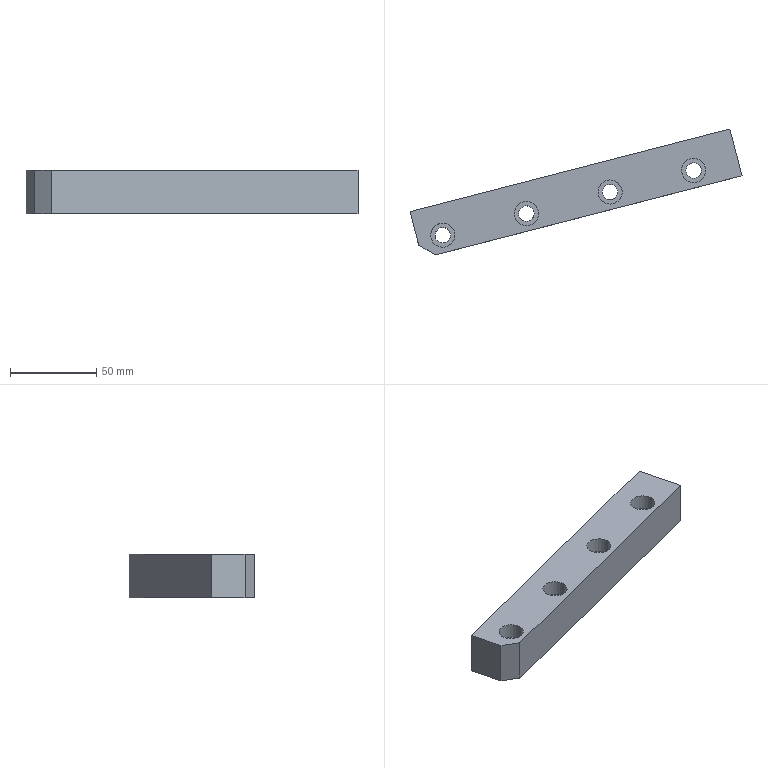Part | STEP file | 车灯-后视镜_id194_x_t | 1 solid | 19 faces | box 192.29 x 72.898 x 25 mm | volume 123539 mm3 | plane 11 | cylinder 8 | commonest cylinder face diameters 9 x4 14 x4
STEP:
#1=CARTESIAN_POINT('',(-276.898,-69.385,-25.286));
#2=VERTEX_POINT('',#1);
#3=CARTESIAN_POINT('',(-278.022,-65.028,-25.286));
#4=DIRECTION('',(0.,0.,1.));
#5=DIRECTION('',(0.2497,-0.9683,0.));
#6=AXIS2_PLACEMENT_3D('',#3,#4,#5);
#7=CIRCLE('',#6,4.5);
#8=EDGE_CURVE('',#2,#2,#7,.T.);
#9=ORIENTED_EDGE('',*,*,#8,.T.);
#10=EDGE_LOOP('',(#9));
#11=FACE_BOUND('',#10,.T.);
#12=CARTESIAN_POINT('',(-325.314,-81.87,-25.286));
#13=VERTEX_POINT('',#12);
#14=CARTESIAN_POINT('',(-326.438,-77.513,-25.286));
#15=DIRECTION('',(0.,0.,1.));
#16=DIRECTION('',(0.2497,-0.9683,0.));
#17=AXIS2_PLACEMENT_3D('',#14,#15,#16);
#18=CIRCLE('',#17,4.5);
#19=EDGE_CURVE('',#13,#13,#18,.T.);
#20=ORIENTED_EDGE('',*,*,#19,.T.);
#21=EDGE_LOOP('',(#20));
#22=FACE_BOUND('',#21,.T.);
#23=CARTESIAN_POINT('',(-373.73,-94.355,-25.286));
#24=VERTEX_POINT('',#23);
#25=CARTESIAN_POINT('',(-374.854,-89.998,-25.286));
#26=DIRECTION('',(0.,0.,1.));
#27=DIRECTION('',(0.2497,-0.9683,0.));
#28=AXIS2_PLACEMENT_3D('',#25,#26,#27);
#29=CIRCLE('',#28,4.5);
#30=EDGE_CURVE('',#24,#24,#29,.T.);
#31=ORIENTED_EDGE('',*,*,#30,.T.);
#32=EDGE_LOOP('',(#31));
#33=FACE_BOUND('',#32,.T.);
#34=CARTESIAN_POINT('',(-422.147,-106.84,-25.286));
#35=VERTEX_POINT('',#34);
#36=CARTESIAN_POINT('',(-423.27,-102.482,-25.286));
#37=DIRECTION('',(0.,0.,1.));
#38=DIRECTION('',(0.2497,-0.9683,0.));
#39=AXIS2_PLACEMENT_3D('',#36,#37,#38);
#40=CIRCLE('',#39,4.5);
#41=EDGE_CURVE('',#35,#35,#40,.T.);
#42=ORIENTED_EDGE('',*,*,#41,.T.);
#43=EDGE_LOOP('',(#42));
#44=FACE_BOUND('',#43,.T.);
#45=CARTESIAN_POINT('',(-250.,-68.129,-25.286));
#46=VERTEX_POINT('',#45);
#47=CARTESIAN_POINT('',(-427.552,-113.914,-25.286));
#48=VERTEX_POINT('',#47);
#49=CARTESIAN_POINT('',(-77.018,-23.523,-25.286));
#50=DIRECTION('',(-0.9683,-0.2497,0.));
#51=VECTOR('',#50,1.);
#52=LINE('',#49,#51);
#53=EDGE_CURVE('',#46,#48,#52,.T.);
#54=ORIENTED_EDGE('',*,*,#53,.T.);
#55=CARTESIAN_POINT('',(-437.296,-108.165,-25.286));
#56=VERTEX_POINT('',#55);
#57=CARTESIAN_POINT('',(-437.296,-108.165,-25.286));
#58=DIRECTION('',(-0.8613,0.5081,0.));
#59=VECTOR('',#58,1.);
#60=LINE('',#57,#59);
#61=EDGE_CURVE('',#48,#56,#60,.T.);
#62=ORIENTED_EDGE('',*,*,#61,.T.);
#63=CARTESIAN_POINT('',(-442.29,-88.798,-25.286));
#64=VERTEX_POINT('',#63);
#65=CARTESIAN_POINT('',(-483.305,70.259,-25.286));
#66=DIRECTION('',(0.2497,-0.9683,0.));
#67=VECTOR('',#66,1.);
#68=LINE('',#65,#67);
#69=EDGE_CURVE('',#64,#56,#68,.T.);
#70=ORIENTED_EDGE('',*,*,#69,.F.);
#71=CARTESIAN_POINT('',(-256.992,-41.016,-25.286));
#72=VERTEX_POINT('',#71);
#73=CARTESIAN_POINT('',(-84.01,3.59,-25.286));
#74=DIRECTION('',(-0.9683,-0.2497,0.));
#75=VECTOR('',#74,1.);
#76=LINE('',#73,#75);
#77=EDGE_CURVE('',#72,#64,#76,.T.);
#78=ORIENTED_EDGE('',*,*,#77,.F.);
#79=CARTESIAN_POINT('',(-256.992,-41.016,-25.286));
#80=DIRECTION('',(0.2497,-0.9683,0.));
#81=VECTOR('',#80,1.);
#82=LINE('',#79,#81);
#83=EDGE_CURVE('',#72,#46,#82,.T.);
#84=ORIENTED_EDGE('',*,*,#83,.T.);
#85=EDGE_LOOP('',(#54,#62,#70,#78,#84));
#86=FACE_BOUND('',#85,.T.);
#87=CARTESIAN_POINT('',(-84.01,3.59,-25.286));
#88=DIRECTION('',(0.,0.,-1.));
#89=DIRECTION('',(-0.9683,-0.2497,0.));
#90=AXIS2_PLACEMENT_3D('',#87,#88,#89);
#91=PLANE('',#90);
#92=ADVANCED_FACE('',(#11,#22,#33,#44,#86),#91,.T.);
#93=ORIENTED_EDGE('',*,*,#69,.T.);
#94=CARTESIAN_POINT('',(-437.296,-108.165,-0.2856));
#95=VERTEX_POINT('',#94);
#96=CARTESIAN_POINT('',(-437.296,-108.165,-100.5));
#97=DIRECTION('',(0.,0.,1.));
#98=VECTOR('',#97,1.);
#99=LINE('',#96,#98);
#100=EDGE_CURVE('',#56,#95,#99,.T.);
#101=ORIENTED_EDGE('',*,*,#100,.T.);
#102=CARTESIAN_POINT('',(-442.29,-88.798,-0.2856));
#103=VERTEX_POINT('',#102);
#104=CARTESIAN_POINT('',(-442.29,-88.798,-0.2856));
#105=DIRECTION('',(0.2497,-0.9683,0.));
#106=VECTOR('',#105,1.);
#107=LINE('',#104,#106);
#108=EDGE_CURVE('',#103,#95,#107,.T.);
#109=ORIENTED_EDGE('',*,*,#108,.F.);
#110=CARTESIAN_POINT('',(-442.29,-88.798,-100.5));
#111=DIRECTION('',(0.,0.,1.));
#112=VECTOR('',#111,1.);
#113=LINE('',#110,#112);
#114=EDGE_CURVE('',#64,#103,#113,.T.);
#115=ORIENTED_EDGE('',*,*,#114,.F.);
#116=EDGE_LOOP('',(#93,#101,#109,#115));
#117=FACE_OUTER_BOUND('',#116,.T.);
#118=CARTESIAN_POINT('',(-483.305,70.259,-100.5));
#119=DIRECTION('',(-0.9683,-0.2497,0.));
#120=DIRECTION('',(0.2497,-0.9683,0.));
#121=AXIS2_PLACEMENT_3D('',#118,#119,#120);
#122=PLANE('',#121);
#123=ADVANCED_FACE('',(#117),#122,.T.);
#124=CARTESIAN_POINT('',(-276.274,-71.806,-0.2856));
#125=VERTEX_POINT('',#124);
#126=CARTESIAN_POINT('',(-278.022,-65.028,-0.2856));
#127=DIRECTION('',(0.,0.,-1.));
#128=DIRECTION('',(0.2497,-0.9683,0.));
#129=AXIS2_PLACEMENT_3D('',#126,#127,#128);
#130=CIRCLE('',#129,7.);
#131=EDGE_CURVE('',#125,#125,#130,.T.);
#132=ORIENTED_EDGE('',*,*,#131,.T.);
#133=EDGE_LOOP('',(#132));
#134=FACE_BOUND('',#133,.T.);
#135=CARTESIAN_POINT('',(-324.69,-84.291,-0.2856));
#136=VERTEX_POINT('',#135);
#137=CARTESIAN_POINT('',(-326.438,-77.513,-0.2856));
#138=DIRECTION('',(0.,0.,-1.));
#139=DIRECTION('',(0.2497,-0.9683,0.));
#140=AXIS2_PLACEMENT_3D('',#137,#138,#139);
#141=CIRCLE('',#140,7.);
#142=EDGE_CURVE('',#136,#136,#141,.T.);
#143=ORIENTED_EDGE('',*,*,#142,.T.);
#144=EDGE_LOOP('',(#143));
#145=FACE_BOUND('',#144,.T.);
#146=CARTESIAN_POINT('',(-373.106,-96.776,-0.2856));
#147=VERTEX_POINT('',#146);
#148=CARTESIAN_POINT('',(-374.854,-89.998,-0.2856));
#149=DIRECTION('',(0.,0.,-1.));
#150=DIRECTION('',(0.2497,-0.9683,0.));
#151=AXIS2_PLACEMENT_3D('',#148,#149,#150);
#152=CIRCLE('',#151,7.);
#153=EDGE_CURVE('',#147,#147,#152,.T.);
#154=ORIENTED_EDGE('',*,*,#153,.T.);
#155=EDGE_LOOP('',(#154));
#156=FACE_BOUND('',#155,.T.);
#157=CARTESIAN_POINT('',(-421.522,-109.261,-0.2856));
#158=VERTEX_POINT('',#157);
#159=CARTESIAN_POINT('',(-423.27,-102.482,-0.2856));
#160=DIRECTION('',(0.,0.,-1.));
#161=DIRECTION('',(0.2497,-0.9683,0.));
#162=AXIS2_PLACEMENT_3D('',#159,#160,#161);
#163=CIRCLE('',#162,7.);
#164=EDGE_CURVE('',#158,#158,#163,.T.);
#165=ORIENTED_EDGE('',*,*,#164,.T.);
#166=EDGE_LOOP('',(#165));
#167=FACE_BOUND('',#166,.T.);
#168=ORIENTED_EDGE('',*,*,#108,.T.);
#169=CARTESIAN_POINT('',(-427.552,-113.914,-0.2856));
#170=VERTEX_POINT('',#169);
#171=CARTESIAN_POINT('',(-437.296,-108.165,-0.2856));
#172=DIRECTION('',(0.8613,-0.5081,0.));
#173=VECTOR('',#172,1.);
#174=LINE('',#171,#173);
#175=EDGE_CURVE('',#95,#170,#174,.T.);
#176=ORIENTED_EDGE('',*,*,#175,.T.);
#177=CARTESIAN_POINT('',(-250.,-68.129,-0.2856));
#178=VERTEX_POINT('',#177);
#179=CARTESIAN_POINT('',(-77.018,-23.523,-0.2856));
#180=DIRECTION('',(-0.9683,-0.2497,0.));
#181=VECTOR('',#180,1.);
#182=LINE('',#179,#181);
#183=EDGE_CURVE('',#178,#170,#182,.T.);
#184=ORIENTED_EDGE('',*,*,#183,.F.);
#185=CARTESIAN_POINT('',(-256.992,-41.016,-0.2856));
#186=VERTEX_POINT('',#185);
#187=CARTESIAN_POINT('',(-256.992,-41.016,-0.2856));
#188=DIRECTION('',(-0.2497,0.9683,0.));
#189=VECTOR('',#188,1.);
#190=LINE('',#187,#189);
#191=EDGE_CURVE('',#178,#186,#190,.T.);
#192=ORIENTED_EDGE('',*,*,#191,.T.);
#193=CARTESIAN_POINT('',(-84.01,3.59,-0.2856));
#194=DIRECTION('',(-0.9683,-0.2497,0.));
#195=VECTOR('',#194,1.);
#196=LINE('',#193,#195);
#197=EDGE_CURVE('',#186,#103,#196,.T.);
#198=ORIENTED_EDGE('',*,*,#197,.T.);
#199=EDGE_LOOP('',(#168,#176,#184,#192,#198));
#200=FACE_BOUND('',#199,.T.);
#201=CARTESIAN_POINT('',(-84.01,3.59,-0.2856));
#202=DIRECTION('',(0.,0.,-1.));
#203=DIRECTION('',(-0.9683,-0.2497,0.));
#204=AXIS2_PLACEMENT_3D('',#201,#202,#203);
#205=PLANE('',#204);
#206=ADVANCED_FACE('',(#134,#145,#156,#167,#200),#205,.F.);
#207=ORIENTED_EDGE('',*,*,#183,.T.);
#208=CARTESIAN_POINT('',(-427.552,-113.914,-25.286));
#209=DIRECTION('',(0.,0.,-1.));
#210=VECTOR('',#209,1.);
#211=LINE('',#208,#210);
#212=EDGE_CURVE('',#170,#48,#211,.T.);
#213=ORIENTED_EDGE('',*,*,#212,.T.);
#214=ORIENTED_EDGE('',*,*,#53,.F.);
#215=CARTESIAN_POINT('',(-250.,-68.129,-25.286));
#216=DIRECTION('',(0.,0.,1.));
#217=VECTOR('',#216,1.);
#218=LINE('',#215,#217);
#219=EDGE_CURVE('',#46,#178,#218,.T.);
#220=ORIENTED_EDGE('',*,*,#219,.T.);
#221=EDGE_LOOP('',(#207,#213,#214,#220));
#222=FACE_OUTER_BOUND('',#221,.T.);
#223=CARTESIAN_POINT('',(-77.018,-23.523,-25.286));
#224=DIRECTION('',(-0.2497,0.9683,0.));
#225=DIRECTION('',(-0.9683,-0.2497,0.));
#226=AXIS2_PLACEMENT_3D('',#223,#224,#225);
#227=PLANE('',#226);
#228=ADVANCED_FACE('',(#222),#227,.F.);
#229=CARTESIAN_POINT('',(-256.992,-41.016,-25.286));
#230=DIRECTION('',(0.,0.,1.));
#231=VECTOR('',#230,1.);
#232=LINE('',#229,#231);
#233=EDGE_CURVE('',#72,#186,#232,.T.);
#234=ORIENTED_EDGE('',*,*,#233,.F.);
#235=ORIENTED_EDGE('',*,*,#77,.T.);
#236=ORIENTED_EDGE('',*,*,#114,.T.);
#237=ORIENTED_EDGE('',*,*,#197,.F.);
#238=EDGE_LOOP('',(#234,#235,#236,#237));
#239=FACE_OUTER_BOUND('',#238,.T.);
#240=CARTESIAN_POINT('',(-84.01,3.59,-25.286));
#241=DIRECTION('',(-0.2497,0.9683,0.));
#242=DIRECTION('',(-0.9683,-0.2497,0.));
#243=AXIS2_PLACEMENT_3D('',#240,#241,#242);
#244=PLANE('',#243);
#245=ADVANCED_FACE('',(#239),#244,.T.);
#246=ORIENTED_EDGE('',*,*,#83,.F.);
#247=ORIENTED_EDGE('',*,*,#233,.T.);
#248=ORIENTED_EDGE('',*,*,#191,.F.);
#249=ORIENTED_EDGE('',*,*,#219,.F.);
#250=EDGE_LOOP('',(#246,#247,#248,#249));
#251=FACE_OUTER_BOUND('',#250,.T.);
#252=CARTESIAN_POINT('',(-250.,-68.129,-0.5));
#253=DIRECTION('',(-0.9683,-0.2497,0.));
#254=DIRECTION('',(0.2497,-0.9683,0.));
#255=AXIS2_PLACEMENT_3D('',#252,#253,#254);
#256=PLANE('',#255);
#257=ADVANCED_FACE('',(#251),#256,.F.);
#258=CARTESIAN_POINT('',(-427.77,-102.482,-9.286));
#259=VERTEX_POINT('',#258);
#260=CARTESIAN_POINT('',(-423.27,-102.482,-9.286));
#261=DIRECTION('',(0.,0.,1.));
#262=DIRECTION('',(-1.,0.,0.));
#263=AXIS2_PLACEMENT_3D('',#260,#261,#262);
#264=CIRCLE('',#263,4.5);
#265=EDGE_CURVE('',#259,#259,#264,.T.);
#266=ORIENTED_EDGE('',*,*,#265,.T.);
#267=EDGE_LOOP('',(#266));
#268=FACE_BOUND('',#267,.T.);
#269=ORIENTED_EDGE('',*,*,#41,.F.);
#270=EDGE_LOOP('',(#269));
#271=FACE_BOUND('',#270,.T.);
#272=CARTESIAN_POINT('',(-423.27,-102.482,-24.786));
#273=DIRECTION('',(0.,0.,1.));
#274=DIRECTION('',(-0.2497,0.9683,0.));
#275=AXIS2_PLACEMENT_3D('',#272,#273,#274);
#276=CYLINDRICAL_SURFACE('',#275,4.5);
#277=ADVANCED_FACE('',(#268,#271),#276,.F.);
#278=ORIENTED_EDGE('',*,*,#265,.F.);
#279=EDGE_LOOP('',(#278));
#280=FACE_BOUND('',#279,.T.);
#281=CARTESIAN_POINT('',(-425.018,-95.704,-9.286));
#282=VERTEX_POINT('',#281);
#283=CARTESIAN_POINT('',(-423.27,-102.482,-9.286));
#284=DIRECTION('',(0.,0.,1.));
#285=DIRECTION('',(-0.2497,0.9683,0.));
#286=AXIS2_PLACEMENT_3D('',#283,#284,#285);
#287=CIRCLE('',#286,7.);
#288=EDGE_CURVE('',#282,#282,#287,.T.);
#289=ORIENTED_EDGE('',*,*,#288,.T.);
#290=EDGE_LOOP('',(#289));
#291=FACE_BOUND('',#290,.T.);
#292=CARTESIAN_POINT('',(-423.27,-102.482,-9.286));
#293=DIRECTION('',(0.,0.,-1.));
#294=DIRECTION('',(0.2497,-0.9683,0.));
#295=AXIS2_PLACEMENT_3D('',#292,#293,#294);
#296=PLANE('',#295);
#297=ADVANCED_FACE('',(#280,#291),#296,.F.);
#298=ORIENTED_EDGE('',*,*,#288,.F.);
#299=EDGE_LOOP('',(#298));
#300=FACE_BOUND('',#299,.T.);
#301=ORIENTED_EDGE('',*,*,#164,.F.);
#302=EDGE_LOOP('',(#301));
#303=FACE_BOUND('',#302,.T.);
#304=CARTESIAN_POINT('',(-423.27,-102.482,-0.2856));
#305=DIRECTION('',(0.,0.,-1.));
#306=DIRECTION('',(0.2497,-0.9683,0.));
#307=AXIS2_PLACEMENT_3D('',#304,#305,#306);
#308=CYLINDRICAL_SURFACE('',#307,7.);
#309=ADVANCED_FACE('',(#300,#303),#308,.F.);
#310=CARTESIAN_POINT('',(-379.354,-89.998,-9.286));
#311=VERTEX_POINT('',#310);
#312=CARTESIAN_POINT('',(-374.854,-89.998,-9.286));
#313=DIRECTION('',(0.,0.,1.));
#314=DIRECTION('',(-1.,0.,0.));
#315=AXIS2_PLACEMENT_3D('',#312,#313,#314);
#316=CIRCLE('',#315,4.5);
#317=EDGE_CURVE('',#311,#311,#316,.T.);
#318=ORIENTED_EDGE('',*,*,#317,.T.);
#319=EDGE_LOOP('',(#318));
#320=FACE_BOUND('',#319,.T.);
#321=ORIENTED_EDGE('',*,*,#30,.F.);
#322=EDGE_LOOP('',(#321));
#323=FACE_BOUND('',#322,.T.);
#324=CARTESIAN_POINT('',(-374.854,-89.998,-24.786));
#325=DIRECTION('',(0.,0.,1.));
#326=DIRECTION('',(-0.2497,0.9683,0.));
#327=AXIS2_PLACEMENT_3D('',#324,#325,#326);
#328=CYLINDRICAL_SURFACE('',#327,4.5);
#329=ADVANCED_FACE('',(#320,#323),#328,.F.);
#330=ORIENTED_EDGE('',*,*,#317,.F.);
#331=EDGE_LOOP('',(#330));
#332=FACE_BOUND('',#331,.T.);
#333=CARTESIAN_POINT('',(-376.602,-83.219,-9.286));
#334=VERTEX_POINT('',#333);
#335=CARTESIAN_POINT('',(-374.854,-89.998,-9.286));
#336=DIRECTION('',(0.,0.,1.));
#337=DIRECTION('',(-0.2497,0.9683,0.));
#338=AXIS2_PLACEMENT_3D('',#335,#336,#337);
#339=CIRCLE('',#338,7.);
#340=EDGE_CURVE('',#334,#334,#339,.T.);
#341=ORIENTED_EDGE('',*,*,#340,.T.);
#342=EDGE_LOOP('',(#341));
#343=FACE_BOUND('',#342,.T.);
#344=CARTESIAN_POINT('',(-374.854,-89.998,-9.286));
#345=DIRECTION('',(0.,0.,-1.));
#346=DIRECTION('',(0.2497,-0.9683,0.));
#347=AXIS2_PLACEMENT_3D('',#344,#345,#346);
#348=PLANE('',#347);
#349=ADVANCED_FACE('',(#332,#343),#348,.F.);
#350=ORIENTED_EDGE('',*,*,#340,.F.);
#351=EDGE_LOOP('',(#350));
#352=FACE_BOUND('',#351,.T.);
#353=ORIENTED_EDGE('',*,*,#153,.F.);
#354=EDGE_LOOP('',(#353));
#355=FACE_BOUND('',#354,.T.);
#356=CARTESIAN_POINT('',(-374.854,-89.998,-0.2856));
#357=DIRECTION('',(0.,0.,-1.));
#358=DIRECTION('',(0.2497,-0.9683,0.));
#359=AXIS2_PLACEMENT_3D('',#356,#357,#358);
#360=CYLINDRICAL_SURFACE('',#359,7.);
#361=ADVANCED_FACE('',(#352,#355),#360,.F.);
#362=CARTESIAN_POINT('',(-330.938,-77.513,-9.286));
#363=VERTEX_POINT('',#362);
#364=CARTESIAN_POINT('',(-326.438,-77.513,-9.286));
#365=DIRECTION('',(0.,0.,1.));
#366=DIRECTION('',(-1.,0.,0.));
#367=AXIS2_PLACEMENT_3D('',#364,#365,#366);
#368=CIRCLE('',#367,4.5);
#369=EDGE_CURVE('',#363,#363,#368,.T.);
#370=ORIENTED_EDGE('',*,*,#369,.T.);
#371=EDGE_LOOP('',(#370));
#372=FACE_BOUND('',#371,.T.);
#373=ORIENTED_EDGE('',*,*,#19,.F.);
#374=EDGE_LOOP('',(#373));
#375=FACE_BOUND('',#374,.T.);
#376=CARTESIAN_POINT('',(-326.438,-77.513,-24.786));
#377=DIRECTION('',(0.,0.,1.));
#378=DIRECTION('',(-0.2497,0.9683,0.));
#379=AXIS2_PLACEMENT_3D('',#376,#377,#378);
#380=CYLINDRICAL_SURFACE('',#379,4.5);
#381=ADVANCED_FACE('',(#372,#375),#380,.F.);
#382=ORIENTED_EDGE('',*,*,#369,.F.);
#383=EDGE_LOOP('',(#382));
#384=FACE_BOUND('',#383,.T.);
#385=CARTESIAN_POINT('',(-328.186,-70.734,-9.286));
#386=VERTEX_POINT('',#385);
#387=CARTESIAN_POINT('',(-326.438,-77.513,-9.286));
#388=DIRECTION('',(0.,0.,1.));
#389=DIRECTION('',(-0.2497,0.9683,0.));
#390=AXIS2_PLACEMENT_3D('',#387,#388,#389);
#391=CIRCLE('',#390,7.);
#392=EDGE_CURVE('',#386,#386,#391,.T.);
#393=ORIENTED_EDGE('',*,*,#392,.T.);
#394=EDGE_LOOP('',(#393));
#395=FACE_BOUND('',#394,.T.);
#396=CARTESIAN_POINT('',(-326.438,-77.513,-9.286));
#397=DIRECTION('',(0.,0.,-1.));
#398=DIRECTION('',(0.2497,-0.9683,0.));
#399=AXIS2_PLACEMENT_3D('',#396,#397,#398);
#400=PLANE('',#399);
#401=ADVANCED_FACE('',(#384,#395),#400,.F.);
#402=ORIENTED_EDGE('',*,*,#392,.F.);
#403=EDGE_LOOP('',(#402));
#404=FACE_BOUND('',#403,.T.);
#405=ORIENTED_EDGE('',*,*,#142,.F.);
#406=EDGE_LOOP('',(#405));
#407=FACE_BOUND('',#406,.T.);
#408=CARTESIAN_POINT('',(-326.438,-77.513,-0.2856));
#409=DIRECTION('',(0.,0.,-1.));
#410=DIRECTION('',(0.2497,-0.9683,0.));
#411=AXIS2_PLACEMENT_3D('',#408,#409,#410);
#412=CYLINDRICAL_SURFACE('',#411,7.);
#413=ADVANCED_FACE('',(#404,#407),#412,.F.);
#414=CARTESIAN_POINT('',(-282.522,-65.028,-9.286));
#415=VERTEX_POINT('',#414);
#416=CARTESIAN_POINT('',(-278.022,-65.028,-9.286));
#417=DIRECTION('',(0.,0.,1.));
#418=DIRECTION('',(-1.,0.,0.));
#419=AXIS2_PLACEMENT_3D('',#416,#417,#418);
#420=CIRCLE('',#419,4.5);
#421=EDGE_CURVE('',#415,#415,#420,.T.);
#422=ORIENTED_EDGE('',*,*,#421,.T.);
#423=EDGE_LOOP('',(#422));
#424=FACE_BOUND('',#423,.T.);
#425=ORIENTED_EDGE('',*,*,#8,.F.);
#426=EDGE_LOOP('',(#425));
#427=FACE_BOUND('',#426,.T.);
#428=CARTESIAN_POINT('',(-278.022,-65.028,-24.786));
#429=DIRECTION('',(0.,0.,1.));
#430=DIRECTION('',(-0.2497,0.9683,0.));
#431=AXIS2_PLACEMENT_3D('',#428,#429,#430);
#432=CYLINDRICAL_SURFACE('',#431,4.5);
#433=ADVANCED_FACE('',(#424,#427),#432,.F.);
#434=ORIENTED_EDGE('',*,*,#421,.F.);
#435=EDGE_LOOP('',(#434));
#436=FACE_BOUND('',#435,.T.);
#437=CARTESIAN_POINT('',(-279.77,-58.249,-9.286));
#438=VERTEX_POINT('',#437);
#439=CARTESIAN_POINT('',(-278.022,-65.028,-9.286));
#440=DIRECTION('',(0.,0.,1.));
#441=DIRECTION('',(-0.2497,0.9683,0.));
#442=AXIS2_PLACEMENT_3D('',#439,#440,#441);
#443=CIRCLE('',#442,7.);
#444=EDGE_CURVE('',#438,#438,#443,.T.);
#445=ORIENTED_EDGE('',*,*,#444,.T.);
#446=EDGE_LOOP('',(#445));
#447=FACE_BOUND('',#446,.T.);
#448=CARTESIAN_POINT('',(-278.022,-65.028,-9.286));
#449=DIRECTION('',(0.,0.,-1.));
#450=DIRECTION('',(0.2497,-0.9683,0.));
#451=AXIS2_PLACEMENT_3D('',#448,#449,#450);
#452=PLANE('',#451);
#453=ADVANCED_FACE('',(#436,#447),#452,.F.);
#454=ORIENTED_EDGE('',*,*,#444,.F.);
#455=EDGE_LOOP('',(#454));
#456=FACE_BOUND('',#455,.T.);
#457=ORIENTED_EDGE('',*,*,#131,.F.);
#458=EDGE_LOOP('',(#457));
#459=FACE_BOUND('',#458,.T.);
#460=CARTESIAN_POINT('',(-278.022,-65.028,-0.2856));
#461=DIRECTION('',(0.,0.,-1.));
#462=DIRECTION('',(0.2497,-0.9683,0.));
#463=AXIS2_PLACEMENT_3D('',#460,#461,#462);
#464=CYLINDRICAL_SURFACE('',#463,7.);
#465=ADVANCED_FACE('',(#456,#459),#464,.F.);
#466=ORIENTED_EDGE('',*,*,#61,.F.);
#467=ORIENTED_EDGE('',*,*,#212,.F.);
#468=ORIENTED_EDGE('',*,*,#175,.F.);
#469=ORIENTED_EDGE('',*,*,#100,.F.);
#470=EDGE_LOOP('',(#466,#467,#468,#469));
#471=FACE_OUTER_BOUND('',#470,.T.);
#472=CARTESIAN_POINT('',(-437.296,-108.165,-100.5));
#473=DIRECTION('',(-0.5081,-0.8613,0.));
#474=DIRECTION('',(0.8613,-0.5081,0.));
#475=AXIS2_PLACEMENT_3D('',#472,#473,#474);
#476=PLANE('',#475);
#477=ADVANCED_FACE('',(#471),#476,.T.);
#478=CLOSED_SHELL('',(#92,#123,#206,#228,#245,#257,#277,#297,#309,#329,#349,#361,#381,#401,#413,#433,#453,#465,#477));
#479=MANIFOLD_SOLID_BREP('',#478);
#480=(LENGTH_UNIT()NAMED_UNIT(*)SI_UNIT(.MILLI.,.METRE.));
#481=UNCERTAINTY_MEASURE_WITH_UNIT(LENGTH_MEASURE(0.00002),#480,'','');
#482=(NAMED_UNIT(*)PLANE_ANGLE_UNIT()SI_UNIT($,.RADIAN.));
#483=PLANE_ANGLE_MEASURE_WITH_UNIT(PLANE_ANGLE_MEASURE(0.01745),#482);
#484=DIMENSIONAL_EXPONENTS(0.,0.,0.,0.,0.,0.,0.);
#485=(CONVERSION_BASED_UNIT('DEGREE',#483)NAMED_UNIT(#484)PLANE_ANGLE_UNIT());
#486=(NAMED_UNIT(*)SI_UNIT($,.STERADIAN.)SOLID_ANGLE_UNIT());
#487=(GEOMETRIC_REPRESENTATION_CONTEXT(3)GLOBAL_UNCERTAINTY_ASSIGNED_CONTEXT((#481))GLOBAL_UNIT_ASSIGNED_CONTEXT((#480,#485,#486))REPRESENTATION_CONTEXT('',''));
#488=ADVANCED_BREP_SHAPE_REPRESENTATION('',(#479),#487);